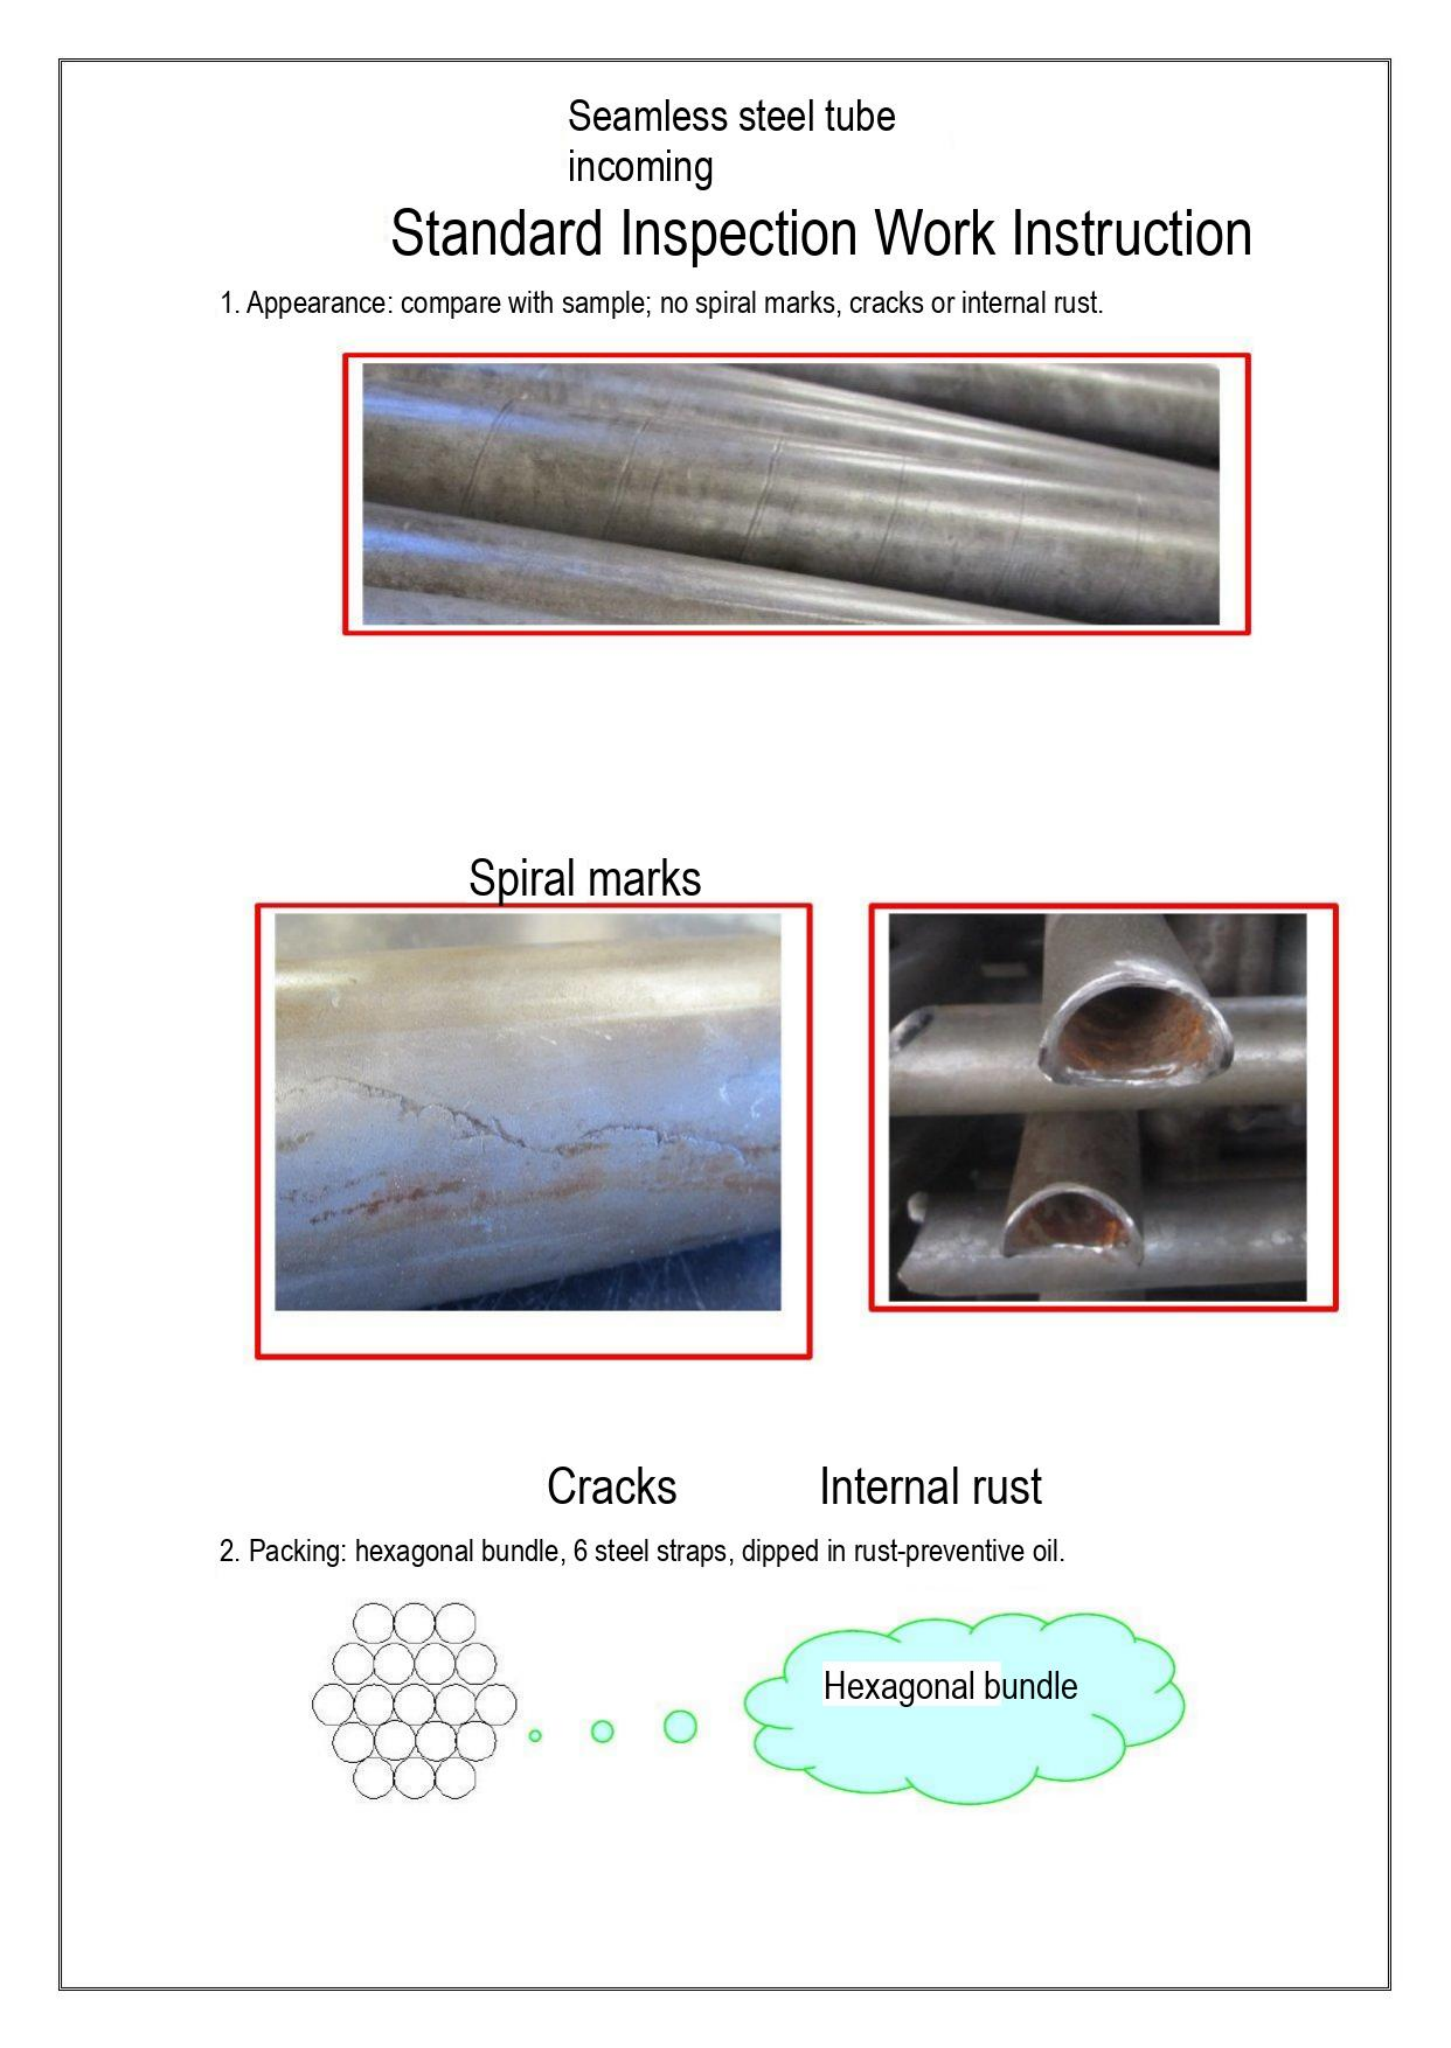Seamless steel tube
incoming
Standard Inspection Work Instruction

1. Appearance: compare with sample; no spiral marks, cracks or internal rust.

Spiral marks

Cracks Internal rust

2. Packing: hexagonal bundle, 6 steel straps, dipped in rust-preventive oil.

Hexagonal bundle
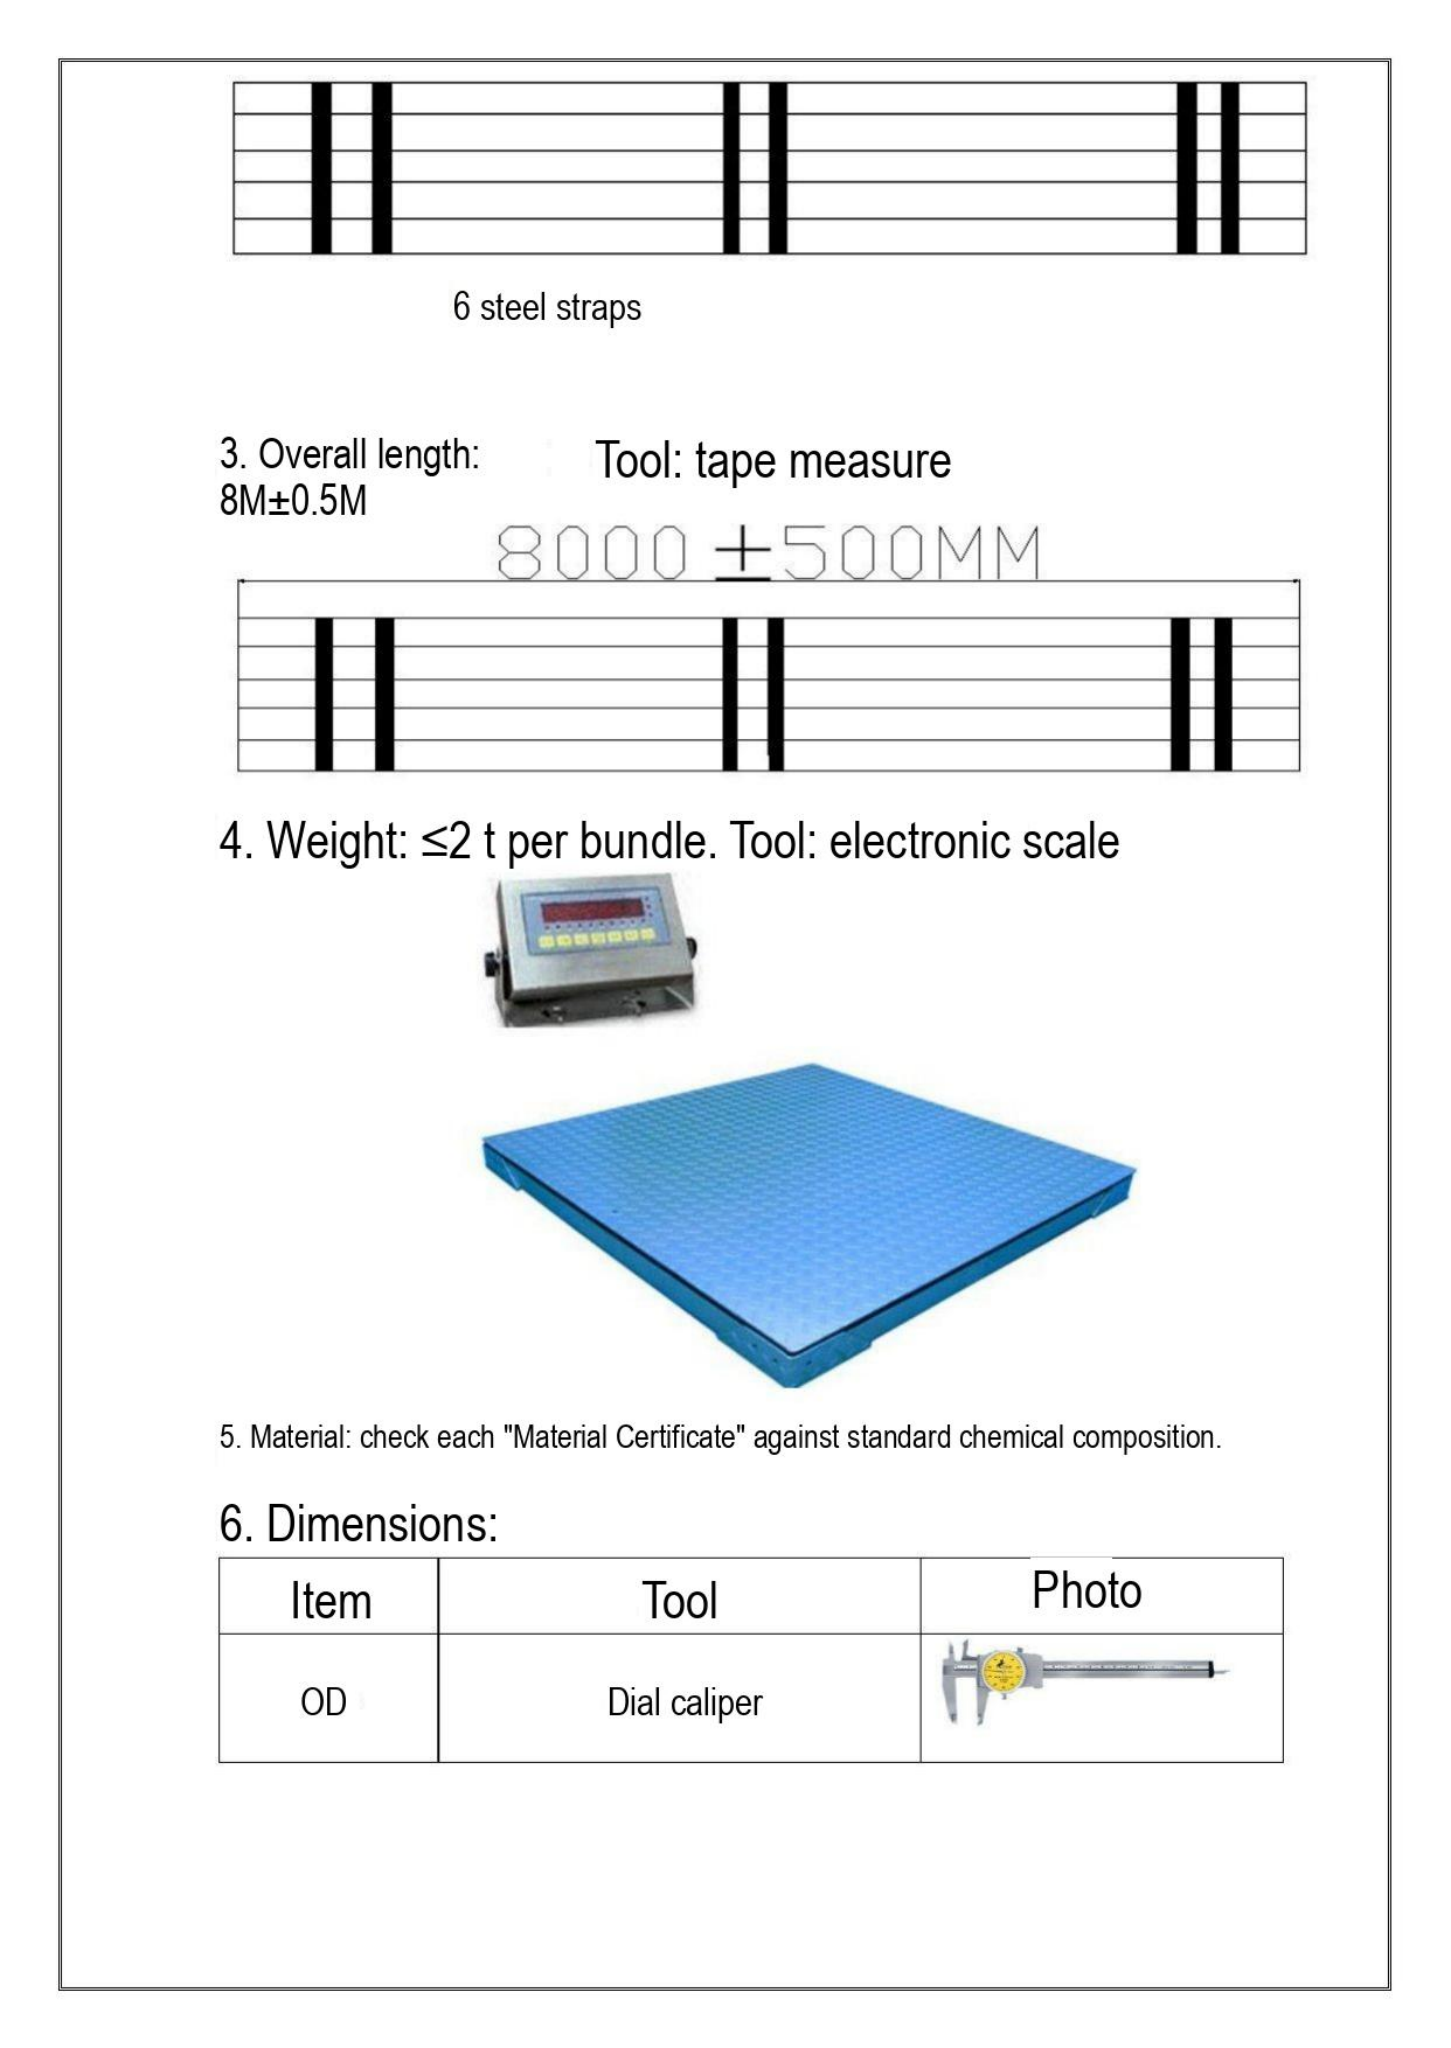6 steel straps

3. Overall length:
8M±0.5M

Tool: tape measure

8000 ±500MM

4. Weight: ≤2 t per bundle. Tool: electronic scale

5. Material: check each "Material Certificate" against standard chemical composition.

6. Dimensions:

| Item | Tool | Photo |
|---|---|---|
| OD | Dial caliper | |
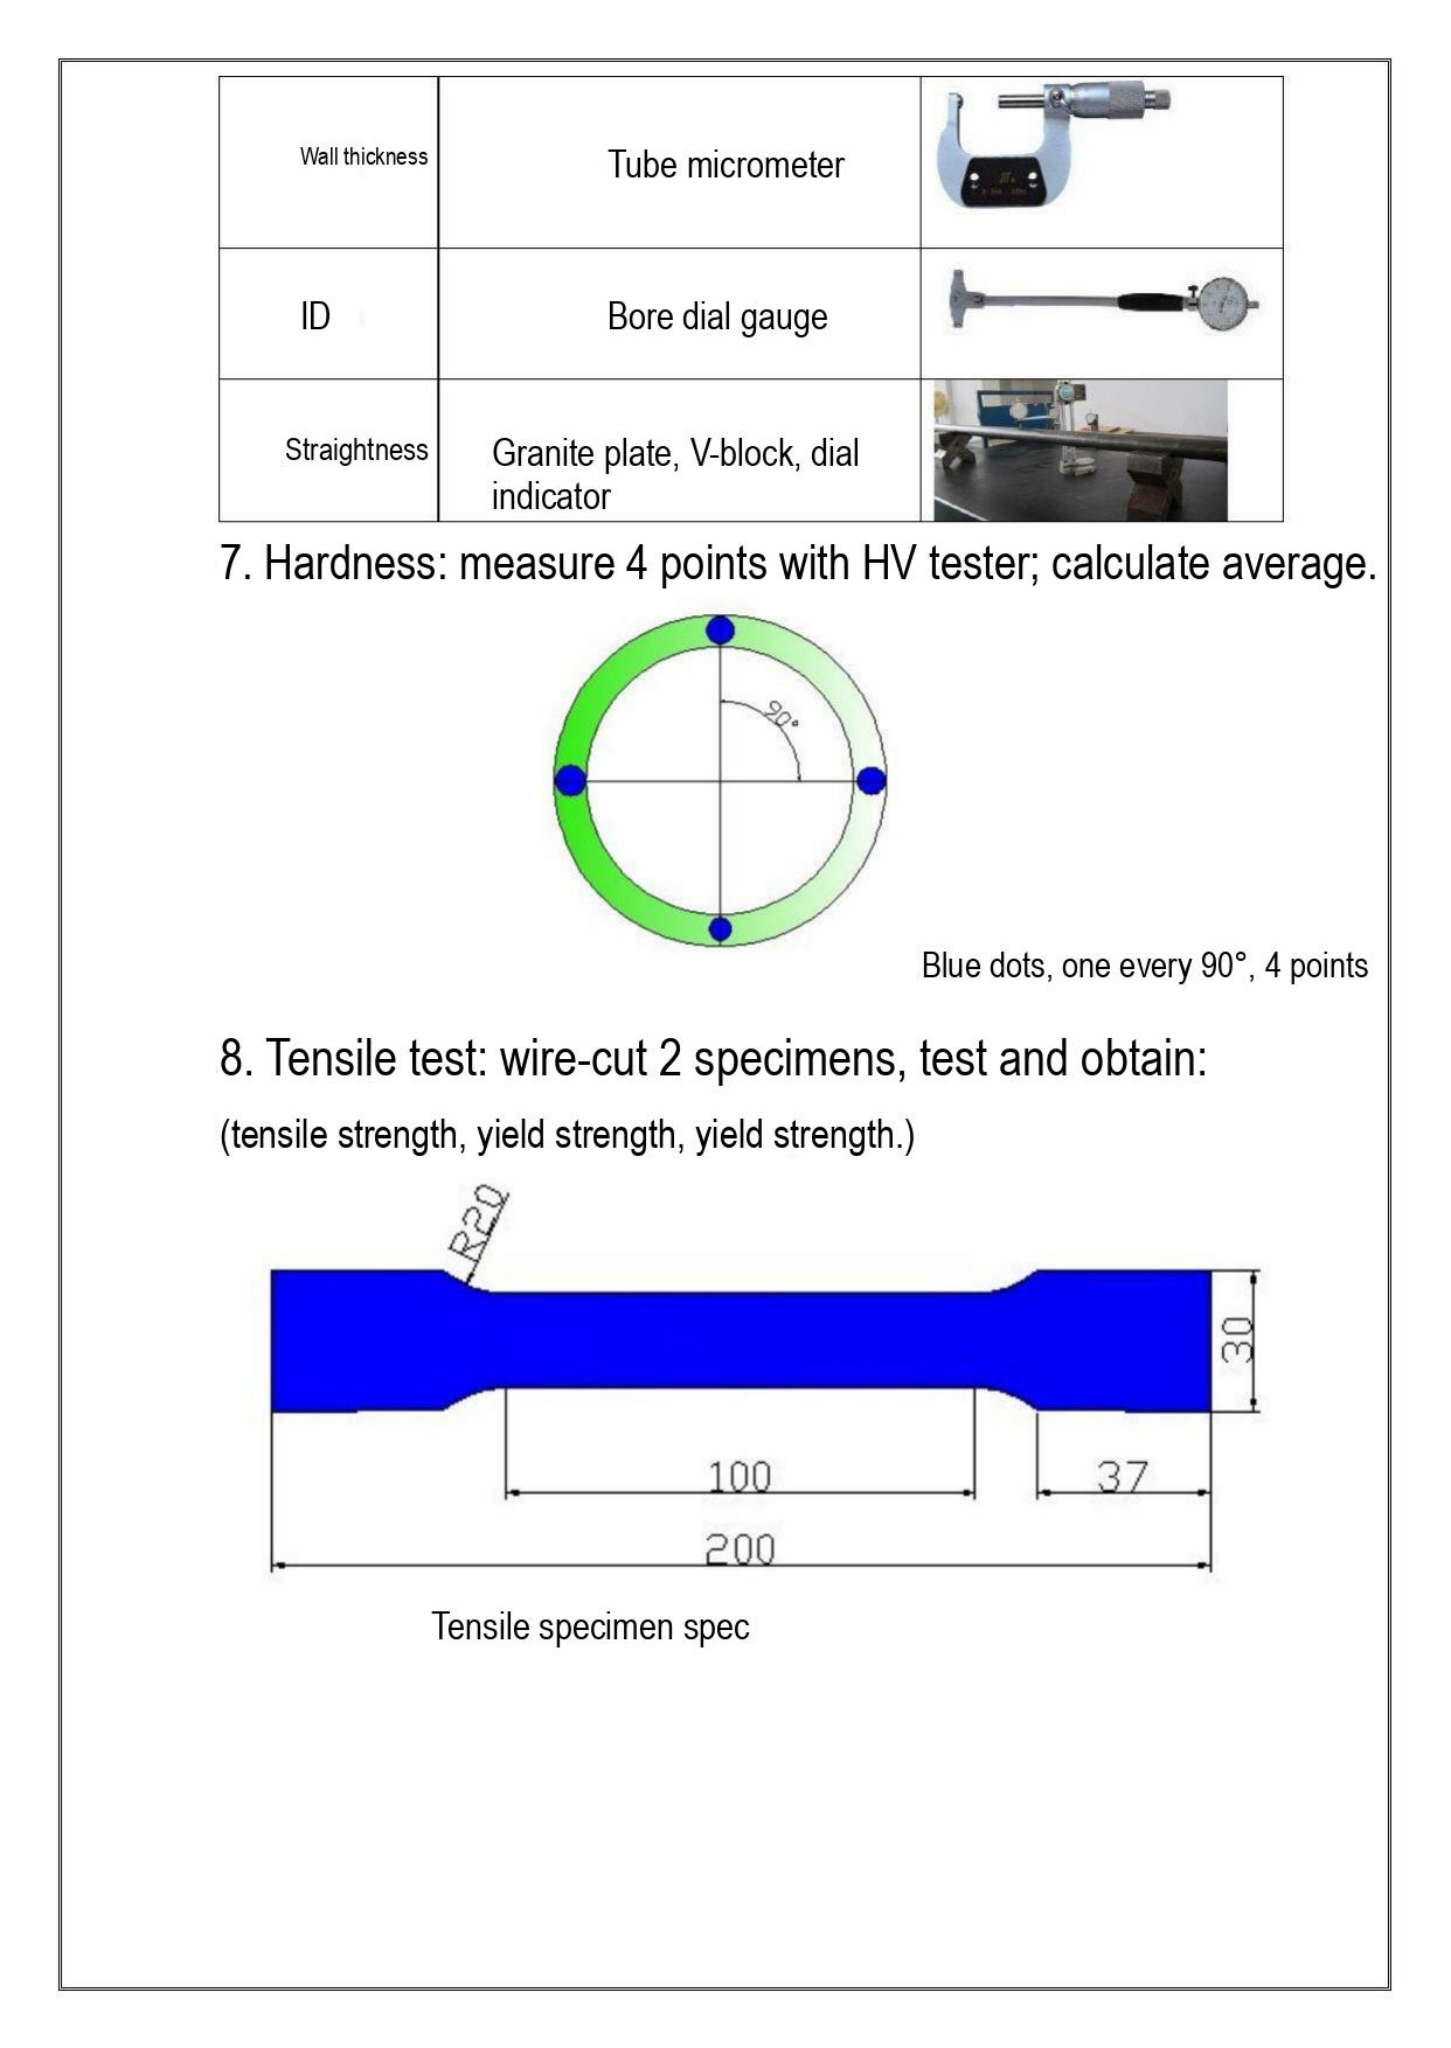| | | |
|---|---|---|
| Wall thickness | Tube micrometer | |
| ID | Bore dial gauge | |
| Straightness | Granite plate, V-block, dial indicator | |

7. Hardness: measure 4 points with HV tester; calculate average.

90°

Blue dots, one every 90°, 4 points

8. Tensile test: wire-cut 2 specimens, test and obtain:

(tensile strength, yield strength, yield strength.)

R20

30

100

37

200

Tensile specimen spec
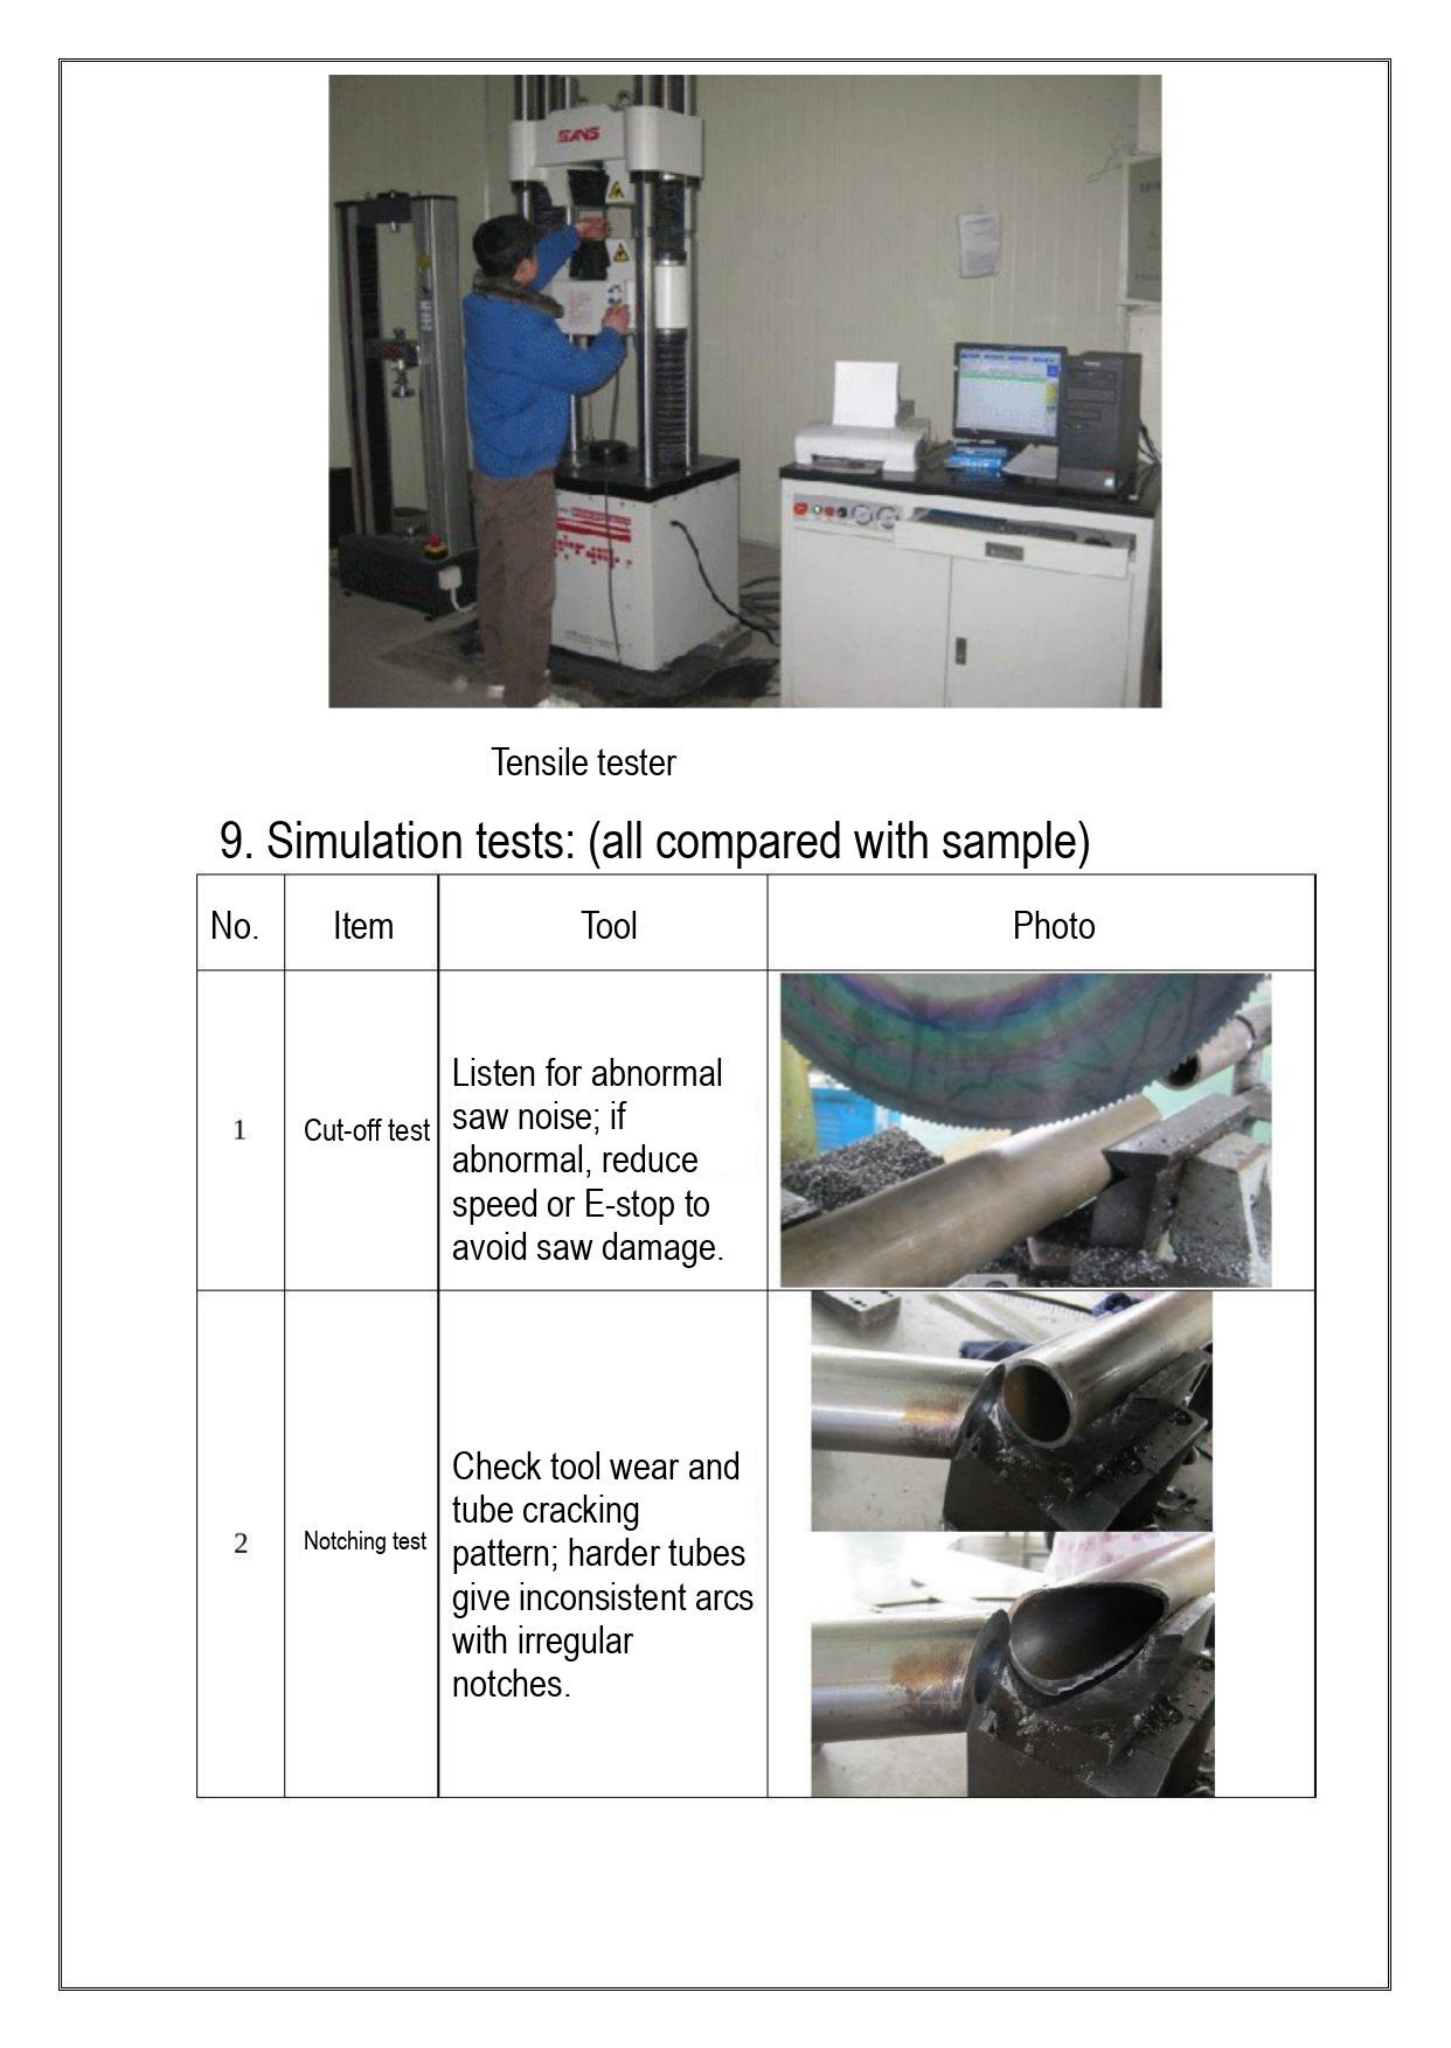SANS

Tensile tester

9. Simulation tests: (all compared with sample)

| No. | Item | Tool | Photo |
|---|---|---|---|
| 1 | Cut-off test | Listen for abnormal saw noise; if abnormal, reduce speed or E-stop to avoid saw damage. | |
| 2 | Notching test | Check tool wear and tube cracking pattern; harder tubes give inconsistent arcs with irregular notches. | |
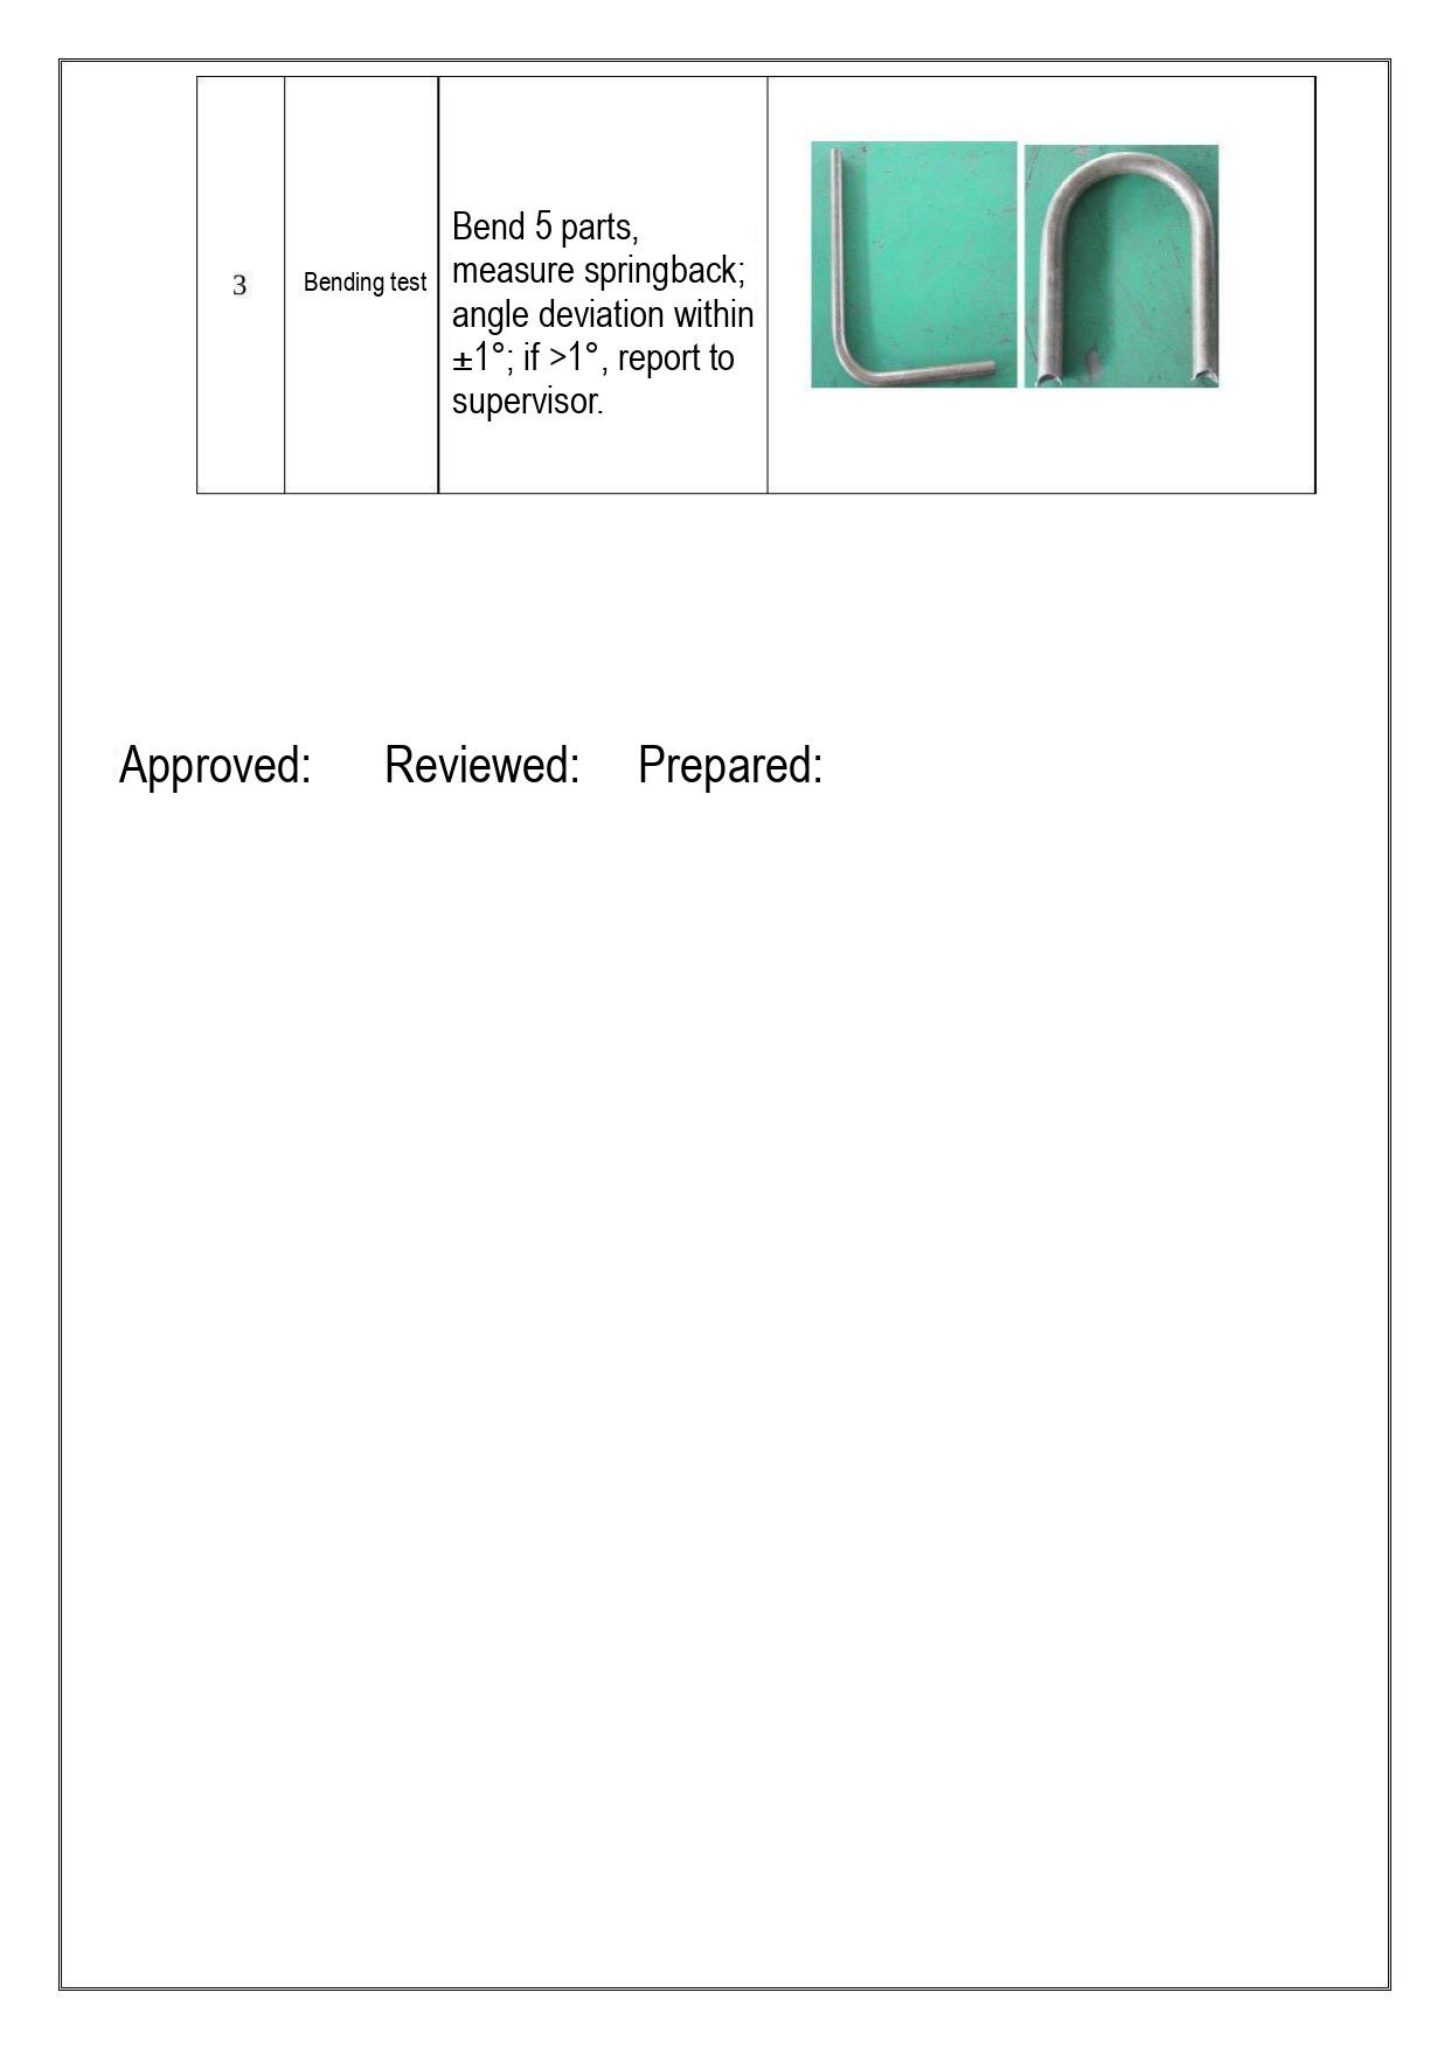| | | | |
|---|---|---|---|
| 3 | Bending test | Bend 5 parts, measure springback; angle deviation within ±1°; if >1°, report to supervisor. | |

Approved: Reviewed: Prepared: